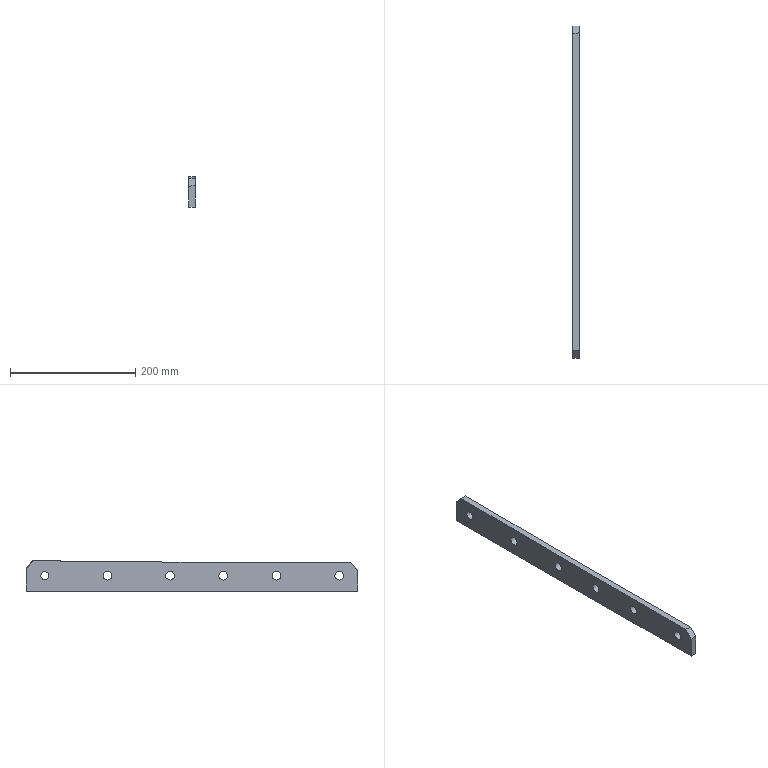Part | NX | features solid 2 | 1 solid | 14 faces | box 10 x 530.061 x 48.788 mm | volume 237252 mm3 | cylinder 6 | plane 5 | spline 3 | commonest cylinder face diameters 14 x5 13 x1
STEP:
#1=CARTESIAN_POINT('',(385.,-179.966,-104.));
#2=VERTEX_POINT('',#1);
#3=CARTESIAN_POINT('',(385.,-179.966,-97.));
#4=DIRECTION('',(1.,0.,0.));
#5=DIRECTION('',(0.,0.,-1.));
#6=AXIS2_PLACEMENT_3D('',#3,#4,#5);
#7=CIRCLE('',#6,7.);
#8=EDGE_CURVE('',#2,#2,#7,.F.);
#9=ORIENTED_EDGE('',*,*,#8,.F.);
#10=EDGE_LOOP('',(#9));
#11=FACE_BOUND('',#10,.T.);
#12=CARTESIAN_POINT('',(385.,-9.966,-104.));
#13=VERTEX_POINT('',#12);
#14=CARTESIAN_POINT('',(385.,-9.966,-97.));
#15=DIRECTION('',(1.,0.,0.));
#16=DIRECTION('',(0.,0.,-1.));
#17=AXIS2_PLACEMENT_3D('',#14,#15,#16);
#18=CIRCLE('',#17,7.);
#19=EDGE_CURVE('',#13,#13,#18,.F.);
#20=ORIENTED_EDGE('',*,*,#19,.F.);
#21=EDGE_LOOP('',(#20));
#22=FACE_BOUND('',#21,.T.);
#23=CARTESIAN_POINT('',(385.,190.034,-103.5));
#24=VERTEX_POINT('',#23);
#25=CARTESIAN_POINT('',(385.,190.034,-97.));
#26=DIRECTION('',(1.,0.,0.));
#27=DIRECTION('',(0.,0.,-1.));
#28=AXIS2_PLACEMENT_3D('',#25,#26,#27);
#29=CIRCLE('',#28,6.5);
#30=EDGE_CURVE('',#24,#24,#29,.F.);
#31=ORIENTED_EDGE('',*,*,#30,.F.);
#32=EDGE_LOOP('',(#31));
#33=FACE_BOUND('',#32,.T.);
#34=CARTESIAN_POINT('',(385.,-310.027,-122.));
#35=VERTEX_POINT('',#34);
#36=CARTESIAN_POINT('',(385.,-310.027,-88.671));
#37=VERTEX_POINT('',#36);
#38=CARTESIAN_POINT('',(385.,-310.027,-52.002));
#39=DIRECTION('',(0.,0.,1.));
#40=VECTOR('',#39,1000.);
#41=LINE('',#38,#40);
#42=EDGE_CURVE('',#35,#37,#41,.T.);
#43=ORIENTED_EDGE('',*,*,#42,.T.);
#44=CARTESIAN_POINT('',(385.,-297.41,-75.971));
#45=VERTEX_POINT('',#44);
#46=CARTESIAN_POINT('',(385.,-310.027,-88.671));
#47=CARTESIAN_POINT('',(385.,-305.821,-84.438));
#48=CARTESIAN_POINT('',(385.,-301.616,-80.204));
#49=CARTESIAN_POINT('',(385.,-297.41,-75.971));
#50=B_SPLINE_CURVE_WITH_KNOTS('',3,(#46,#47,#48,#49),.UNSPECIFIED.,.F.,.F.,(4,4),(0.,1.002),.UNSPECIFIED.);
#51=EDGE_CURVE('',#37,#45,#50,.T.);
#52=ORIENTED_EDGE('',*,*,#51,.T.);
#53=CARTESIAN_POINT('',(385.,207.794,-73.23));
#54=VERTEX_POINT('',#53);
#55=CARTESIAN_POINT('',(385.,-297.41,-75.971));
#56=CARTESIAN_POINT('',(385.,-129.004,-76.3));
#57=CARTESIAN_POINT('',(385.,39.406,-75.701));
#58=CARTESIAN_POINT('',(385.,207.794,-73.23));
#59=B_SPLINE_CURVE_WITH_KNOTS('',3,(#55,#56,#57,#58),.UNSPECIFIED.,.F.,.F.,(4,4),(0.,0.5052),.UNSPECIFIED.);
#60=EDGE_CURVE('',#45,#54,#59,.T.);
#61=ORIENTED_EDGE('',*,*,#60,.T.);
#62=CARTESIAN_POINT('',(385.,220.034,-85.37));
#63=VERTEX_POINT('',#62);
#64=CARTESIAN_POINT('',(385.,207.794,-73.23));
#65=CARTESIAN_POINT('',(385.,211.874,-77.277));
#66=CARTESIAN_POINT('',(385.,215.954,-81.323));
#67=CARTESIAN_POINT('',(385.,220.034,-85.37));
#68=B_SPLINE_CURVE_WITH_KNOTS('',3,(#64,#65,#66,#67),.UNSPECIFIED.,.F.,.F.,(4,4),(0.,1.),.UNSPECIFIED.);
#69=EDGE_CURVE('',#54,#63,#68,.T.);
#70=ORIENTED_EDGE('',*,*,#69,.T.);
#71=CARTESIAN_POINT('',(385.,220.034,-122.));
#72=VERTEX_POINT('',#71);
#73=CARTESIAN_POINT('',(385.,220.034,-79.38));
#74=DIRECTION('',(0.,0.,-1.));
#75=VECTOR('',#74,1000.);
#76=LINE('',#73,#75);
#77=EDGE_CURVE('',#63,#72,#76,.T.);
#78=ORIENTED_EDGE('',*,*,#77,.T.);
#79=CARTESIAN_POINT('',(385.,5.001,-122.));
#80=DIRECTION('',(0.,1.,0.));
#81=VECTOR('',#80,1000.);
#82=LINE('',#79,#81);
#83=EDGE_CURVE('',#35,#72,#82,.T.);
#84=ORIENTED_EDGE('',*,*,#83,.F.);
#85=EDGE_LOOP('',(#43,#52,#61,#70,#78,#84));
#86=FACE_BOUND('',#85,.T.);
#87=CARTESIAN_POINT('',(385.,90.034,-104.));
#88=VERTEX_POINT('',#87);
#89=CARTESIAN_POINT('',(385.,90.034,-97.));
#90=DIRECTION('',(1.,0.,0.));
#91=DIRECTION('',(0.,0.,-1.));
#92=AXIS2_PLACEMENT_3D('',#89,#90,#91);
#93=CIRCLE('',#92,7.);
#94=EDGE_CURVE('',#88,#88,#93,.F.);
#95=ORIENTED_EDGE('',*,*,#94,.F.);
#96=EDGE_LOOP('',(#95));
#97=FACE_BOUND('',#96,.T.);
#98=CARTESIAN_POINT('',(385.,-94.966,-104.));
#99=VERTEX_POINT('',#98);
#100=CARTESIAN_POINT('',(385.,-94.966,-97.));
#101=DIRECTION('',(1.,0.,0.));
#102=DIRECTION('',(0.,0.,-1.));
#103=AXIS2_PLACEMENT_3D('',#100,#101,#102);
#104=CIRCLE('',#103,7.);
#105=EDGE_CURVE('',#99,#99,#104,.F.);
#106=ORIENTED_EDGE('',*,*,#105,.F.);
#107=EDGE_LOOP('',(#106));
#108=FACE_BOUND('',#107,.T.);
#109=CARTESIAN_POINT('',(385.,-279.966,-104.));
#110=VERTEX_POINT('',#109);
#111=CARTESIAN_POINT('',(385.,-279.966,-97.));
#112=DIRECTION('',(1.,0.,0.));
#113=DIRECTION('',(0.,0.,-1.));
#114=AXIS2_PLACEMENT_3D('',#111,#112,#113);
#115=CIRCLE('',#114,7.);
#116=EDGE_CURVE('',#110,#110,#115,.F.);
#117=ORIENTED_EDGE('',*,*,#116,.F.);
#118=EDGE_LOOP('',(#117));
#119=FACE_BOUND('',#118,.T.);
#120=CARTESIAN_POINT('',(385.,5.001,-79.38));
#121=DIRECTION('',(1.,0.,0.));
#122=DIRECTION('',(0.,0.,1.));
#123=AXIS2_PLACEMENT_3D('',#120,#121,#122);
#124=PLANE('',#123);
#125=ADVANCED_FACE('',(#11,#22,#33,#86,#97,#108,#119),#124,.F.);
#126=CARTESIAN_POINT('',(395.,-179.966,-104.));
#127=VERTEX_POINT('',#126);
#128=CARTESIAN_POINT('',(395.,-179.966,-97.));
#129=DIRECTION('',(1.,0.,0.));
#130=DIRECTION('',(0.,0.,-1.));
#131=AXIS2_PLACEMENT_3D('',#128,#129,#130);
#132=CIRCLE('',#131,7.);
#133=EDGE_CURVE('',#127,#127,#132,.T.);
#134=ORIENTED_EDGE('',*,*,#133,.F.);
#135=EDGE_LOOP('',(#134));
#136=FACE_BOUND('',#135,.T.);
#137=CARTESIAN_POINT('',(395.,-9.966,-104.));
#138=VERTEX_POINT('',#137);
#139=CARTESIAN_POINT('',(395.,-9.966,-97.));
#140=DIRECTION('',(1.,0.,0.));
#141=DIRECTION('',(0.,0.,-1.));
#142=AXIS2_PLACEMENT_3D('',#139,#140,#141);
#143=CIRCLE('',#142,7.);
#144=EDGE_CURVE('',#138,#138,#143,.T.);
#145=ORIENTED_EDGE('',*,*,#144,.F.);
#146=EDGE_LOOP('',(#145));
#147=FACE_BOUND('',#146,.T.);
#148=CARTESIAN_POINT('',(395.,190.034,-103.5));
#149=VERTEX_POINT('',#148);
#150=CARTESIAN_POINT('',(395.,190.034,-97.));
#151=DIRECTION('',(1.,0.,0.));
#152=DIRECTION('',(0.,0.,-1.));
#153=AXIS2_PLACEMENT_3D('',#150,#151,#152);
#154=CIRCLE('',#153,6.5);
#155=EDGE_CURVE('',#149,#149,#154,.T.);
#156=ORIENTED_EDGE('',*,*,#155,.F.);
#157=EDGE_LOOP('',(#156));
#158=FACE_BOUND('',#157,.T.);
#159=CARTESIAN_POINT('',(395.,-298.73,-75.968));
#160=VERTEX_POINT('',#159);
#161=CARTESIAN_POINT('',(395.,209.065,-73.212));
#162=VERTEX_POINT('',#161);
#163=CARTESIAN_POINT('',(395.,-298.73,-75.968));
#164=CARTESIAN_POINT('',(395.,-214.095,-76.134));
#165=CARTESIAN_POINT('',(395.,-44.825,-76.053));
#166=CARTESIAN_POINT('',(395.,124.439,-74.454));
#167=CARTESIAN_POINT('',(395.,209.065,-73.212));
#168=B_SPLINE_CURVE_WITH_KNOTS('',3,(#163,#164,#165,#166,#167),.UNSPECIFIED.,.F.,.F.,(4,1,4),(0.,0.2539,0.5078),.UNSPECIFIED.);
#169=EDGE_CURVE('',#160,#162,#168,.T.);
#170=ORIENTED_EDGE('',*,*,#169,.F.);
#171=CARTESIAN_POINT('',(395.,-310.027,-87.351));
#172=VERTEX_POINT('',#171);
#173=CARTESIAN_POINT('',(395.,-298.73,-75.968));
#174=CARTESIAN_POINT('',(395.,-302.496,-79.762));
#175=CARTESIAN_POINT('',(395.,-306.261,-83.557));
#176=CARTESIAN_POINT('',(395.,-310.027,-87.351));
#177=B_SPLINE_CURVE_WITH_KNOTS('',3,(#173,#174,#175,#176),.UNSPECIFIED.,.F.,.F.,(4,4),(0.03993,1.),.UNSPECIFIED.);
#178=EDGE_CURVE('',#160,#172,#177,.T.);
#179=ORIENTED_EDGE('',*,*,#178,.T.);
#180=CARTESIAN_POINT('',(395.,-310.027,-122.));
#181=VERTEX_POINT('',#180);
#182=CARTESIAN_POINT('',(395.,-310.027,-52.002));
#183=DIRECTION('',(0.,0.,1.));
#184=VECTOR('',#183,1000.);
#185=LINE('',#182,#184);
#186=EDGE_CURVE('',#181,#172,#185,.T.);
#187=ORIENTED_EDGE('',*,*,#186,.F.);
#188=CARTESIAN_POINT('',(395.,220.034,-122.));
#189=VERTEX_POINT('',#188);
#190=CARTESIAN_POINT('',(395.,5.001,-122.));
#191=DIRECTION('',(0.,1.,0.));
#192=VECTOR('',#191,1000.);
#193=LINE('',#190,#192);
#194=EDGE_CURVE('',#181,#189,#193,.T.);
#195=ORIENTED_EDGE('',*,*,#194,.T.);
#196=CARTESIAN_POINT('',(395.,220.034,-84.101));
#197=VERTEX_POINT('',#196);
#198=CARTESIAN_POINT('',(395.,220.034,-75.181));
#199=DIRECTION('',(0.,0.,-1.));
#200=VECTOR('',#199,1000.);
#201=LINE('',#198,#200);
#202=EDGE_CURVE('',#197,#189,#201,.T.);
#203=ORIENTED_EDGE('',*,*,#202,.F.);
#204=CARTESIAN_POINT('',(395.,220.034,-84.101));
#205=CARTESIAN_POINT('',(395.,216.378,-80.471));
#206=CARTESIAN_POINT('',(395.,212.721,-76.841));
#207=CARTESIAN_POINT('',(395.,209.065,-73.212));
#208=B_SPLINE_CURVE_WITH_KNOTS('',3,(#204,#205,#206,#207),.UNSPECIFIED.,.F.,.F.,(4,4),(0.,0.9381),.UNSPECIFIED.);
#209=EDGE_CURVE('',#197,#162,#208,.T.);
#210=ORIENTED_EDGE('',*,*,#209,.T.);
#211=EDGE_LOOP('',(#170,#179,#187,#195,#203,#210));
#212=FACE_BOUND('',#211,.T.);
#213=CARTESIAN_POINT('',(395.,90.034,-104.));
#214=VERTEX_POINT('',#213);
#215=CARTESIAN_POINT('',(395.,90.034,-97.));
#216=DIRECTION('',(1.,0.,0.));
#217=DIRECTION('',(0.,0.,-1.));
#218=AXIS2_PLACEMENT_3D('',#215,#216,#217);
#219=CIRCLE('',#218,7.);
#220=EDGE_CURVE('',#214,#214,#219,.T.);
#221=ORIENTED_EDGE('',*,*,#220,.F.);
#222=EDGE_LOOP('',(#221));
#223=FACE_BOUND('',#222,.T.);
#224=CARTESIAN_POINT('',(395.,-94.966,-104.));
#225=VERTEX_POINT('',#224);
#226=CARTESIAN_POINT('',(395.,-94.966,-97.));
#227=DIRECTION('',(1.,0.,0.));
#228=DIRECTION('',(0.,0.,-1.));
#229=AXIS2_PLACEMENT_3D('',#226,#227,#228);
#230=CIRCLE('',#229,7.);
#231=EDGE_CURVE('',#225,#225,#230,.T.);
#232=ORIENTED_EDGE('',*,*,#231,.F.);
#233=EDGE_LOOP('',(#232));
#234=FACE_BOUND('',#233,.T.);
#235=CARTESIAN_POINT('',(395.,-279.966,-104.));
#236=VERTEX_POINT('',#235);
#237=CARTESIAN_POINT('',(395.,-279.966,-97.));
#238=DIRECTION('',(1.,0.,0.));
#239=DIRECTION('',(0.,0.,-1.));
#240=AXIS2_PLACEMENT_3D('',#237,#238,#239);
#241=CIRCLE('',#240,7.);
#242=EDGE_CURVE('',#236,#236,#241,.T.);
#243=ORIENTED_EDGE('',*,*,#242,.F.);
#244=EDGE_LOOP('',(#243));
#245=FACE_BOUND('',#244,.T.);
#246=CARTESIAN_POINT('',(395.,5.001,-75.181));
#247=DIRECTION('',(1.,0.,0.));
#248=DIRECTION('',(0.,0.,1.));
#249=AXIS2_PLACEMENT_3D('',#246,#247,#248);
#250=PLANE('',#249);
#251=ADVANCED_FACE('',(#136,#147,#158,#212,#223,#234,#245),#250,.T.);
#252=ORIENTED_EDGE('',*,*,#155,.T.);
#253=EDGE_LOOP('',(#252));
#254=FACE_BOUND('',#253,.T.);
#255=ORIENTED_EDGE('',*,*,#30,.T.);
#256=EDGE_LOOP('',(#255));
#257=FACE_BOUND('',#256,.T.);
#258=CARTESIAN_POINT('',(365.,190.034,-97.));
#259=DIRECTION('',(1.,0.,0.));
#260=DIRECTION('',(0.,0.,1.));
#261=AXIS2_PLACEMENT_3D('',#258,#259,#260);
#262=CYLINDRICAL_SURFACE('',#261,6.5);
#263=ADVANCED_FACE('',(#254,#257),#262,.F.);
#264=ORIENTED_EDGE('',*,*,#83,.T.);
#265=CARTESIAN_POINT('',(54.5,220.034,-122.));
#266=DIRECTION('',(-1.,0.,0.));
#267=VECTOR('',#266,1000.);
#268=LINE('',#265,#267);
#269=EDGE_CURVE('',#189,#72,#268,.T.);
#270=ORIENTED_EDGE('',*,*,#269,.F.);
#271=ORIENTED_EDGE('',*,*,#194,.F.);
#272=CARTESIAN_POINT('',(173.5,-310.027,-122.));
#273=DIRECTION('',(1.,0.,0.));
#274=VECTOR('',#273,1000.);
#275=LINE('',#272,#274);
#276=EDGE_CURVE('',#35,#181,#275,.T.);
#277=ORIENTED_EDGE('',*,*,#276,.F.);
#278=EDGE_LOOP('',(#264,#270,#271,#277));
#279=FACE_BOUND('',#278,.T.);
#280=CARTESIAN_POINT('',(-563.409,-238.872,-122.));
#281=DIRECTION('',(0.,0.,-1.));
#282=DIRECTION('',(1.,0.,0.));
#283=AXIS2_PLACEMENT_3D('',#280,#281,#282);
#284=PLANE('',#283);
#285=ADVANCED_FACE('',(#279),#284,.T.);
#286=ORIENTED_EDGE('',*,*,#77,.F.);
#287=CARTESIAN_POINT('',(395.,220.034,-84.101));
#288=CARTESIAN_POINT('',(391.667,220.034,-84.524));
#289=CARTESIAN_POINT('',(388.333,220.034,-84.947));
#290=CARTESIAN_POINT('',(385.,220.034,-85.37));
#291=B_SPLINE_CURVE_WITH_KNOTS('',3,(#287,#288,#289,#290),.UNSPECIFIED.,.F.,.F.,(4,4),(0.,1.),.UNSPECIFIED.);
#292=EDGE_CURVE('',#63,#197,#291,.F.);
#293=ORIENTED_EDGE('',*,*,#292,.T.);
#294=ORIENTED_EDGE('',*,*,#202,.T.);
#295=ORIENTED_EDGE('',*,*,#269,.T.);
#296=EDGE_LOOP('',(#286,#293,#294,#295));
#297=FACE_BOUND('',#296,.T.);
#298=CARTESIAN_POINT('',(54.5,220.034,-52.002));
#299=DIRECTION('',(0.,1.,0.));
#300=DIRECTION('',(0.,0.,1.));
#301=AXIS2_PLACEMENT_3D('',#298,#299,#300);
#302=PLANE('',#301);
#303=ADVANCED_FACE('',(#297),#302,.T.);
#304=ORIENTED_EDGE('',*,*,#186,.T.);
#305=CARTESIAN_POINT('',(385.,-310.027,-88.671));
#306=CARTESIAN_POINT('',(388.333,-310.027,-88.231));
#307=CARTESIAN_POINT('',(391.667,-310.027,-87.791));
#308=CARTESIAN_POINT('',(395.,-310.027,-87.351));
#309=B_SPLINE_CURVE_WITH_KNOTS('',3,(#305,#306,#307,#308),.UNSPECIFIED.,.F.,.F.,(4,4),(0.,1.),.UNSPECIFIED.);
#310=EDGE_CURVE('',#172,#37,#309,.F.);
#311=ORIENTED_EDGE('',*,*,#310,.T.);
#312=ORIENTED_EDGE('',*,*,#42,.F.);
#313=ORIENTED_EDGE('',*,*,#276,.T.);
#314=EDGE_LOOP('',(#304,#311,#312,#313));
#315=FACE_BOUND('',#314,.T.);
#316=CARTESIAN_POINT('',(173.5,-310.027,-52.002));
#317=DIRECTION('',(0.,-1.,0.));
#318=DIRECTION('',(0.,0.,-1.));
#319=AXIS2_PLACEMENT_3D('',#316,#317,#318);
#320=PLANE('',#319);
#321=ADVANCED_FACE('',(#315),#320,.T.);
#322=ORIENTED_EDGE('',*,*,#60,.F.);
#323=CARTESIAN_POINT('',(385.,-297.409,-75.971));
#324=CARTESIAN_POINT('',(388.335,-297.838,-75.97));
#325=CARTESIAN_POINT('',(391.668,-298.278,-75.969));
#326=CARTESIAN_POINT('',(395.,-298.729,-75.968));
#327=B_SPLINE_CURVE_WITH_KNOTS('',3,(#323,#324,#325,#326),.UNSPECIFIED.,.F.,.F.,(4,4),(0.,0.01009),.UNSPECIFIED.);
#328=EDGE_CURVE('',#45,#160,#327,.T.);
#329=ORIENTED_EDGE('',*,*,#328,.T.);
#330=ORIENTED_EDGE('',*,*,#169,.T.);
#331=CARTESIAN_POINT('',(395.,209.064,-73.212));
#332=CARTESIAN_POINT('',(391.668,208.632,-73.218));
#333=CARTESIAN_POINT('',(388.335,208.208,-73.224));
#334=CARTESIAN_POINT('',(385.,207.793,-73.23));
#335=B_SPLINE_CURVE_WITH_KNOTS('',3,(#331,#332,#333,#334),.UNSPECIFIED.,.F.,.F.,(4,4),(0.,0.01008),.UNSPECIFIED.);
#336=EDGE_CURVE('',#162,#54,#335,.T.);
#337=ORIENTED_EDGE('',*,*,#336,.T.);
#338=EDGE_LOOP('',(#322,#329,#330,#337));
#339=FACE_BOUND('',#338,.T.);
#340=CARTESIAN_POINT('',(385.,-301.777,-75.962));
#341=CARTESIAN_POINT('',(395.06,-301.777,-75.962));
#342=CARTESIAN_POINT('',(385.,-216.126,-76.13));
#343=CARTESIAN_POINT('',(395.06,-216.126,-76.13));
#344=CARTESIAN_POINT('',(385.,-44.823,-76.07));
#345=CARTESIAN_POINT('',(395.06,-44.823,-76.07));
#346=CARTESIAN_POINT('',(385.,126.471,-74.424));
#347=CARTESIAN_POINT('',(395.06,126.471,-74.424));
#348=CARTESIAN_POINT('',(385.,212.111,-73.167));
#349=CARTESIAN_POINT('',(395.06,212.111,-73.167));
#350=B_SPLINE_SURFACE_WITH_KNOTS('',3,1,((#340,#341),(#342,#343),(#344,#345),(#346,#347),(#348,#349)),.SURF_OF_LINEAR_EXTRUSION.,.F.,.F.,.F.,(4,1,4),(2,2),(-0.008645,0.5,1.009),(0.,1.),.UNSPECIFIED.);
#351=ADVANCED_FACE('',(#339),#350,.F.);
#352=ORIENTED_EDGE('',*,*,#220,.T.);
#353=EDGE_LOOP('',(#352));
#354=FACE_BOUND('',#353,.T.);
#355=ORIENTED_EDGE('',*,*,#94,.T.);
#356=EDGE_LOOP('',(#355));
#357=FACE_BOUND('',#356,.T.);
#358=CARTESIAN_POINT('',(365.,90.034,-97.));
#359=DIRECTION('',(1.,0.,0.));
#360=DIRECTION('',(0.,0.,1.));
#361=AXIS2_PLACEMENT_3D('',#358,#359,#360);
#362=CYLINDRICAL_SURFACE('',#361,7.);
#363=ADVANCED_FACE('',(#354,#357),#362,.F.);
#364=ORIENTED_EDGE('',*,*,#144,.T.);
#365=EDGE_LOOP('',(#364));
#366=FACE_BOUND('',#365,.T.);
#367=ORIENTED_EDGE('',*,*,#19,.T.);
#368=EDGE_LOOP('',(#367));
#369=FACE_BOUND('',#368,.T.);
#370=CARTESIAN_POINT('',(365.,-9.966,-97.));
#371=DIRECTION('',(1.,0.,0.));
#372=DIRECTION('',(0.,0.,1.));
#373=AXIS2_PLACEMENT_3D('',#370,#371,#372);
#374=CYLINDRICAL_SURFACE('',#373,7.);
#375=ADVANCED_FACE('',(#366,#369),#374,.F.);
#376=ORIENTED_EDGE('',*,*,#231,.T.);
#377=EDGE_LOOP('',(#376));
#378=FACE_BOUND('',#377,.T.);
#379=ORIENTED_EDGE('',*,*,#105,.T.);
#380=EDGE_LOOP('',(#379));
#381=FACE_BOUND('',#380,.T.);
#382=CARTESIAN_POINT('',(365.,-94.966,-97.));
#383=DIRECTION('',(1.,0.,0.));
#384=DIRECTION('',(0.,0.,1.));
#385=AXIS2_PLACEMENT_3D('',#382,#383,#384);
#386=CYLINDRICAL_SURFACE('',#385,7.);
#387=ADVANCED_FACE('',(#378,#381),#386,.F.);
#388=ORIENTED_EDGE('',*,*,#133,.T.);
#389=EDGE_LOOP('',(#388));
#390=FACE_BOUND('',#389,.T.);
#391=ORIENTED_EDGE('',*,*,#8,.T.);
#392=EDGE_LOOP('',(#391));
#393=FACE_BOUND('',#392,.T.);
#394=CARTESIAN_POINT('',(365.,-179.966,-97.));
#395=DIRECTION('',(1.,0.,0.));
#396=DIRECTION('',(0.,0.,1.));
#397=AXIS2_PLACEMENT_3D('',#394,#395,#396);
#398=CYLINDRICAL_SURFACE('',#397,7.);
#399=ADVANCED_FACE('',(#390,#393),#398,.F.);
#400=ORIENTED_EDGE('',*,*,#242,.T.);
#401=EDGE_LOOP('',(#400));
#402=FACE_BOUND('',#401,.T.);
#403=ORIENTED_EDGE('',*,*,#116,.T.);
#404=EDGE_LOOP('',(#403));
#405=FACE_BOUND('',#404,.T.);
#406=CARTESIAN_POINT('',(365.,-279.966,-97.));
#407=DIRECTION('',(1.,0.,0.));
#408=DIRECTION('',(0.,0.,1.));
#409=AXIS2_PLACEMENT_3D('',#406,#407,#408);
#410=CYLINDRICAL_SURFACE('',#409,7.);
#411=ADVANCED_FACE('',(#402,#405),#410,.F.);
#412=ORIENTED_EDGE('',*,*,#51,.F.);
#413=ORIENTED_EDGE('',*,*,#310,.F.);
#414=ORIENTED_EDGE('',*,*,#178,.F.);
#415=ORIENTED_EDGE('',*,*,#328,.F.);
#416=EDGE_LOOP('',(#412,#413,#414,#415));
#417=FACE_BOUND('',#416,.T.);
#418=CARTESIAN_POINT('',(383.318,-297.333,-76.111));
#419=CARTESIAN_POINT('',(387.172,-297.333,-75.617));
#420=CARTESIAN_POINT('',(391.027,-297.333,-75.105));
#421=CARTESIAN_POINT('',(394.88,-297.333,-74.578));
#422=CARTESIAN_POINT('',(384.931,-310.027,-88.68));
#423=CARTESIAN_POINT('',(388.821,-310.027,-88.181));
#424=CARTESIAN_POINT('',(392.71,-310.027,-87.665));
#425=CARTESIAN_POINT('',(396.597,-310.027,-87.133));
#426=B_SPLINE_SURFACE_WITH_KNOTS('',1,3,((#418,#419,#420,#421),(#422,#423,#424,#425)),.RULED_SURF.,.F.,.F.,.F.,(2,2),(4,4),(0.492,1.),(0.1308,0.1426),.PIECEWISE_BEZIER_KNOTS.);
#427=ADVANCED_FACE('',(#417),#426,.T.);
#428=ORIENTED_EDGE('',*,*,#209,.F.);
#429=ORIENTED_EDGE('',*,*,#292,.F.);
#430=ORIENTED_EDGE('',*,*,#69,.F.);
#431=ORIENTED_EDGE('',*,*,#336,.F.);
#432=EDGE_LOOP('',(#428,#429,#430,#431));
#433=FACE_BOUND('',#432,.T.);
#434=CARTESIAN_POINT('',(394.898,207.722,-71.894));
#435=CARTESIAN_POINT('',(391.079,207.721,-72.392));
#436=CARTESIAN_POINT('',(387.259,207.72,-72.878));
#437=CARTESIAN_POINT('',(383.439,207.72,-73.352));
#438=CARTESIAN_POINT('',(396.464,220.034,-83.91));
#439=CARTESIAN_POINT('',(392.621,220.034,-84.411));
#440=CARTESIAN_POINT('',(388.777,220.034,-84.901));
#441=CARTESIAN_POINT('',(384.932,220.034,-85.378));
#442=B_SPLINE_SURFACE_WITH_KNOTS('',1,3,((#434,#435,#436,#437),(#438,#439,#440,#441)),.RULED_SURF.,.F.,.F.,.F.,(2,2),(4,4),(0.5067,1.),(0.09614,0.1078),.PIECEWISE_BEZIER_KNOTS.);
#443=ADVANCED_FACE('',(#433),#442,.T.);
#444=CLOSED_SHELL('',(#125,#251,#263,#285,#303,#321,#351,#363,#375,#387,#399,#411,#427,#443));
#445=MANIFOLD_SOLID_BREP('',#444);
#446=(LENGTH_UNIT()NAMED_UNIT(*)SI_UNIT(.MILLI.,.METRE.));
#447=UNCERTAINTY_MEASURE_WITH_UNIT(LENGTH_MEASURE(0.1016),#446,'','');
#448=(NAMED_UNIT(*)PLANE_ANGLE_UNIT()SI_UNIT($,.RADIAN.));
#449=(NAMED_UNIT(*)SI_UNIT($,.STERADIAN.)SOLID_ANGLE_UNIT());
#450=(GEOMETRIC_REPRESENTATION_CONTEXT(3)GLOBAL_UNCERTAINTY_ASSIGNED_CONTEXT((#447))GLOBAL_UNIT_ASSIGNED_CONTEXT((#446,#448,#449))REPRESENTATION_CONTEXT('',''));
#451=ADVANCED_BREP_SHAPE_REPRESENTATION('',(#445),#450);